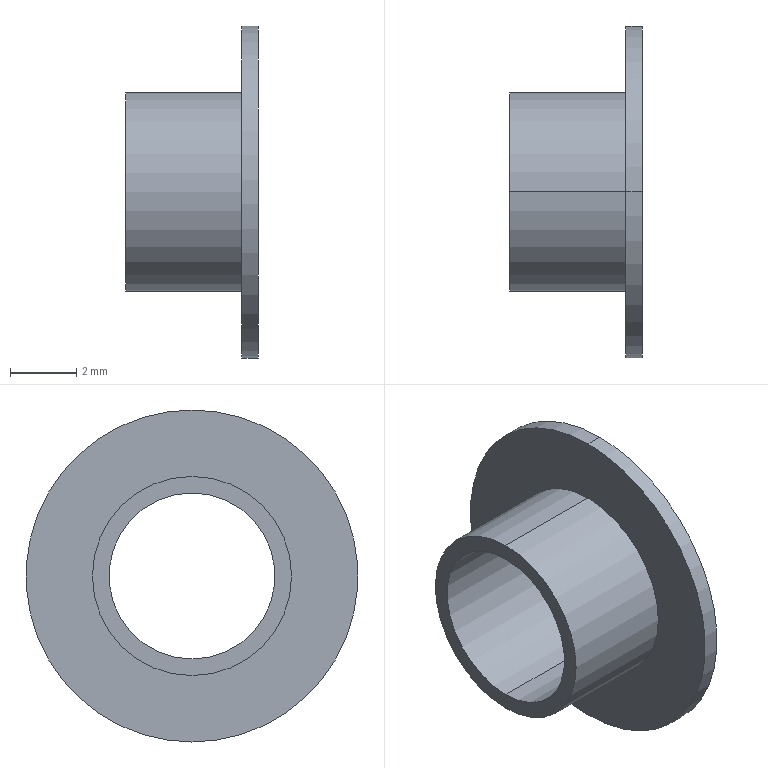Part | SolidWorks | features Revolution 1 | 1 solid | 9 faces | box 4 x 10 x 10 mm | volume 59.69 mm3 | cylinder 6 | plane 3 | commonest cylinder face diameters 5 x2 6 x2 10 x2
STEP:
#1=CARTESIAN_POINT('',(4.,0.,5.));
#2=VERTEX_POINT('',#1);
#3=CARTESIAN_POINT('',(4.,0.,-5.));
#4=VERTEX_POINT('',#3);
#5=CARTESIAN_POINT('',(4.,0.,0.));
#6=DIRECTION('',(-1.,0.,0.));
#7=DIRECTION('',(0.,0.,1.));
#8=AXIS2_PLACEMENT_3D('',#5,#6,#7);
#9=CIRCLE('',#8,5.);
#10=EDGE_CURVE('',#2,#4,#9,.T.);
#11=ORIENTED_EDGE('',*,*,#10,.T.);
#12=CARTESIAN_POINT('',(3.5,0.,-5.));
#13=VERTEX_POINT('',#12);
#14=CARTESIAN_POINT('',(-238.363,0.,-5.));
#15=DIRECTION('',(-1.,0.,0.));
#16=VECTOR('',#15,1000.);
#17=LINE('',#14,#16);
#18=EDGE_CURVE('',#4,#13,#17,.T.);
#19=ORIENTED_EDGE('',*,*,#18,.T.);
#20=CARTESIAN_POINT('',(3.5,0.,5.));
#21=VERTEX_POINT('',#20);
#22=CARTESIAN_POINT('',(3.5,0.,0.));
#23=DIRECTION('',(-1.,0.,0.));
#24=DIRECTION('',(0.,0.,1.));
#25=AXIS2_PLACEMENT_3D('',#22,#23,#24);
#26=CIRCLE('',#25,5.);
#27=EDGE_CURVE('',#21,#13,#26,.T.);
#28=ORIENTED_EDGE('',*,*,#27,.F.);
#29=CARTESIAN_POINT('',(-238.363,0.,5.));
#30=DIRECTION('',(-1.,0.,0.));
#31=VECTOR('',#30,1000.);
#32=LINE('',#29,#31);
#33=EDGE_CURVE('',#2,#21,#32,.T.);
#34=ORIENTED_EDGE('',*,*,#33,.F.);
#35=EDGE_LOOP('',(#11,#19,#28,#34));
#36=FACE_OUTER_BOUND('',#35,.T.);
#37=CARTESIAN_POINT('',(-238.363,0.,0.));
#38=DIRECTION('',(-1.,0.,0.));
#39=DIRECTION('',(0.,0.,1.));
#40=AXIS2_PLACEMENT_3D('',#37,#38,#39);
#41=CYLINDRICAL_SURFACE('',#40,5.);
#42=ADVANCED_FACE('',(#36),#41,.T.);
#43=CARTESIAN_POINT('',(3.5,0.,3.));
#44=VERTEX_POINT('',#43);
#45=CARTESIAN_POINT('',(3.5,0.,-3.));
#46=VERTEX_POINT('',#45);
#47=CARTESIAN_POINT('',(3.5,0.,0.));
#48=DIRECTION('',(-1.,0.,0.));
#49=DIRECTION('',(0.,0.,1.));
#50=AXIS2_PLACEMENT_3D('',#47,#48,#49);
#51=CIRCLE('',#50,3.);
#52=EDGE_CURVE('',#44,#46,#51,.T.);
#53=ORIENTED_EDGE('',*,*,#52,.T.);
#54=CARTESIAN_POINT('',(0.,0.,-3.));
#55=VERTEX_POINT('',#54);
#56=CARTESIAN_POINT('',(-238.363,0.,-3.));
#57=DIRECTION('',(-1.,0.,0.));
#58=VECTOR('',#57,1000.);
#59=LINE('',#56,#58);
#60=EDGE_CURVE('',#46,#55,#59,.T.);
#61=ORIENTED_EDGE('',*,*,#60,.T.);
#62=CARTESIAN_POINT('',(0.,0.,3.));
#63=VERTEX_POINT('',#62);
#64=CARTESIAN_POINT('',(0.,0.,0.));
#65=DIRECTION('',(-1.,0.,0.));
#66=DIRECTION('',(0.,0.,1.));
#67=AXIS2_PLACEMENT_3D('',#64,#65,#66);
#68=CIRCLE('',#67,3.);
#69=EDGE_CURVE('',#63,#55,#68,.T.);
#70=ORIENTED_EDGE('',*,*,#69,.F.);
#71=CARTESIAN_POINT('',(-238.363,0.,3.));
#72=DIRECTION('',(-1.,0.,0.));
#73=VECTOR('',#72,1000.);
#74=LINE('',#71,#73);
#75=EDGE_CURVE('',#44,#63,#74,.T.);
#76=ORIENTED_EDGE('',*,*,#75,.F.);
#77=EDGE_LOOP('',(#53,#61,#70,#76));
#78=FACE_OUTER_BOUND('',#77,.T.);
#79=CARTESIAN_POINT('',(-238.363,0.,0.));
#80=DIRECTION('',(-1.,0.,0.));
#81=DIRECTION('',(0.,0.,1.));
#82=AXIS2_PLACEMENT_3D('',#79,#80,#81);
#83=CYLINDRICAL_SURFACE('',#82,3.);
#84=ADVANCED_FACE('',(#78),#83,.T.);
#85=CARTESIAN_POINT('',(4.,0.,-2.5));
#86=VERTEX_POINT('',#85);
#87=CARTESIAN_POINT('',(4.,0.,2.5));
#88=VERTEX_POINT('',#87);
#89=CARTESIAN_POINT('',(4.,0.,0.));
#90=DIRECTION('',(-1.,0.,0.));
#91=DIRECTION('',(0.,0.,1.));
#92=AXIS2_PLACEMENT_3D('',#89,#90,#91);
#93=CIRCLE('',#92,2.5);
#94=EDGE_CURVE('',#86,#88,#93,.T.);
#95=ORIENTED_EDGE('',*,*,#94,.F.);
#96=CARTESIAN_POINT('',(0.,0.,-2.5));
#97=VERTEX_POINT('',#96);
#98=CARTESIAN_POINT('',(-238.363,0.,-2.5));
#99=DIRECTION('',(-1.,0.,0.));
#100=VECTOR('',#99,1000.);
#101=LINE('',#98,#100);
#102=EDGE_CURVE('',#86,#97,#101,.T.);
#103=ORIENTED_EDGE('',*,*,#102,.T.);
#104=CARTESIAN_POINT('',(0.,0.,2.5));
#105=VERTEX_POINT('',#104);
#106=CARTESIAN_POINT('',(0.,0.,0.));
#107=DIRECTION('',(-1.,0.,0.));
#108=DIRECTION('',(0.,0.,1.));
#109=AXIS2_PLACEMENT_3D('',#106,#107,#108);
#110=CIRCLE('',#109,2.5);
#111=EDGE_CURVE('',#97,#105,#110,.T.);
#112=ORIENTED_EDGE('',*,*,#111,.T.);
#113=CARTESIAN_POINT('',(-238.363,0.,2.5));
#114=DIRECTION('',(-1.,0.,0.));
#115=VECTOR('',#114,1000.);
#116=LINE('',#113,#115);
#117=EDGE_CURVE('',#88,#105,#116,.T.);
#118=ORIENTED_EDGE('',*,*,#117,.F.);
#119=EDGE_LOOP('',(#95,#103,#112,#118));
#120=FACE_OUTER_BOUND('',#119,.T.);
#121=CARTESIAN_POINT('',(-238.363,0.,0.));
#122=DIRECTION('',(-1.,0.,0.));
#123=DIRECTION('',(0.,0.,1.));
#124=AXIS2_PLACEMENT_3D('',#121,#122,#123);
#125=CYLINDRICAL_SURFACE('',#124,2.5);
#126=ADVANCED_FACE('',(#120),#125,.F.);
#127=ORIENTED_EDGE('',*,*,#102,.F.);
#128=CARTESIAN_POINT('',(4.,0.,0.));
#129=DIRECTION('',(-1.,0.,0.));
#130=DIRECTION('',(0.,0.,1.));
#131=AXIS2_PLACEMENT_3D('',#128,#129,#130);
#132=CIRCLE('',#131,2.5);
#133=EDGE_CURVE('',#88,#86,#132,.T.);
#134=ORIENTED_EDGE('',*,*,#133,.F.);
#135=ORIENTED_EDGE('',*,*,#117,.T.);
#136=CARTESIAN_POINT('',(0.,0.,0.));
#137=DIRECTION('',(-1.,0.,0.));
#138=DIRECTION('',(0.,0.,1.));
#139=AXIS2_PLACEMENT_3D('',#136,#137,#138);
#140=CIRCLE('',#139,2.5);
#141=EDGE_CURVE('',#105,#97,#140,.T.);
#142=ORIENTED_EDGE('',*,*,#141,.T.);
#143=EDGE_LOOP('',(#127,#134,#135,#142));
#144=FACE_OUTER_BOUND('',#143,.T.);
#145=CARTESIAN_POINT('',(-238.363,0.,0.));
#146=DIRECTION('',(-1.,0.,0.));
#147=DIRECTION('',(0.,0.,1.));
#148=AXIS2_PLACEMENT_3D('',#145,#146,#147);
#149=CYLINDRICAL_SURFACE('',#148,2.5);
#150=ADVANCED_FACE('',(#144),#149,.F.);
#151=ORIENTED_EDGE('',*,*,#141,.F.);
#152=ORIENTED_EDGE('',*,*,#111,.F.);
#153=EDGE_LOOP('',(#151,#152));
#154=FACE_BOUND('',#153,.T.);
#155=ORIENTED_EDGE('',*,*,#69,.T.);
#156=CARTESIAN_POINT('',(0.,0.,0.));
#157=DIRECTION('',(-1.,0.,0.));
#158=DIRECTION('',(0.,0.,1.));
#159=AXIS2_PLACEMENT_3D('',#156,#157,#158);
#160=CIRCLE('',#159,3.);
#161=EDGE_CURVE('',#55,#63,#160,.T.);
#162=ORIENTED_EDGE('',*,*,#161,.T.);
#163=EDGE_LOOP('',(#155,#162));
#164=FACE_OUTER_BOUND('',#163,.T.);
#165=CARTESIAN_POINT('',(0.,0.,-2.5));
#166=DIRECTION('',(1.,0.,0.));
#167=DIRECTION('',(0.,0.,-1.));
#168=AXIS2_PLACEMENT_3D('',#165,#166,#167);
#169=PLANE('',#168);
#170=ADVANCED_FACE('',(#154,#164),#169,.F.);
#171=ORIENTED_EDGE('',*,*,#60,.F.);
#172=CARTESIAN_POINT('',(3.5,0.,0.));
#173=DIRECTION('',(-1.,0.,0.));
#174=DIRECTION('',(0.,0.,1.));
#175=AXIS2_PLACEMENT_3D('',#172,#173,#174);
#176=CIRCLE('',#175,3.);
#177=EDGE_CURVE('',#46,#44,#176,.T.);
#178=ORIENTED_EDGE('',*,*,#177,.T.);
#179=ORIENTED_EDGE('',*,*,#75,.T.);
#180=ORIENTED_EDGE('',*,*,#161,.F.);
#181=EDGE_LOOP('',(#171,#178,#179,#180));
#182=FACE_OUTER_BOUND('',#181,.T.);
#183=CARTESIAN_POINT('',(-238.363,0.,0.));
#184=DIRECTION('',(-1.,0.,0.));
#185=DIRECTION('',(0.,0.,1.));
#186=AXIS2_PLACEMENT_3D('',#183,#184,#185);
#187=CYLINDRICAL_SURFACE('',#186,3.);
#188=ADVANCED_FACE('',(#182),#187,.T.);
#189=ORIENTED_EDGE('',*,*,#52,.F.);
#190=ORIENTED_EDGE('',*,*,#177,.F.);
#191=EDGE_LOOP('',(#189,#190));
#192=FACE_BOUND('',#191,.T.);
#193=ORIENTED_EDGE('',*,*,#27,.T.);
#194=CARTESIAN_POINT('',(3.5,0.,0.));
#195=DIRECTION('',(-1.,0.,0.));
#196=DIRECTION('',(0.,0.,1.));
#197=AXIS2_PLACEMENT_3D('',#194,#195,#196);
#198=CIRCLE('',#197,5.);
#199=EDGE_CURVE('',#13,#21,#198,.T.);
#200=ORIENTED_EDGE('',*,*,#199,.T.);
#201=EDGE_LOOP('',(#193,#200));
#202=FACE_OUTER_BOUND('',#201,.T.);
#203=CARTESIAN_POINT('',(3.5,0.,-3.));
#204=DIRECTION('',(1.,0.,0.));
#205=DIRECTION('',(0.,0.,-1.));
#206=AXIS2_PLACEMENT_3D('',#203,#204,#205);
#207=PLANE('',#206);
#208=ADVANCED_FACE('',(#192,#202),#207,.F.);
#209=ORIENTED_EDGE('',*,*,#18,.F.);
#210=CARTESIAN_POINT('',(4.,0.,0.));
#211=DIRECTION('',(-1.,0.,0.));
#212=DIRECTION('',(0.,0.,1.));
#213=AXIS2_PLACEMENT_3D('',#210,#211,#212);
#214=CIRCLE('',#213,5.);
#215=EDGE_CURVE('',#4,#2,#214,.T.);
#216=ORIENTED_EDGE('',*,*,#215,.T.);
#217=ORIENTED_EDGE('',*,*,#33,.T.);
#218=ORIENTED_EDGE('',*,*,#199,.F.);
#219=EDGE_LOOP('',(#209,#216,#217,#218));
#220=FACE_OUTER_BOUND('',#219,.T.);
#221=CARTESIAN_POINT('',(-238.363,0.,0.));
#222=DIRECTION('',(-1.,0.,0.));
#223=DIRECTION('',(0.,0.,1.));
#224=AXIS2_PLACEMENT_3D('',#221,#222,#223);
#225=CYLINDRICAL_SURFACE('',#224,5.);
#226=ADVANCED_FACE('',(#220),#225,.T.);
#227=ORIENTED_EDGE('',*,*,#10,.F.);
#228=ORIENTED_EDGE('',*,*,#215,.F.);
#229=EDGE_LOOP('',(#227,#228));
#230=FACE_OUTER_BOUND('',#229,.T.);
#231=ORIENTED_EDGE('',*,*,#133,.T.);
#232=ORIENTED_EDGE('',*,*,#94,.T.);
#233=EDGE_LOOP('',(#231,#232));
#234=FACE_BOUND('',#233,.T.);
#235=CARTESIAN_POINT('',(4.,0.,-5.));
#236=DIRECTION('',(-1.,0.,0.));
#237=DIRECTION('',(0.,0.,1.));
#238=AXIS2_PLACEMENT_3D('',#235,#236,#237);
#239=PLANE('',#238);
#240=ADVANCED_FACE('',(#230,#234),#239,.F.);
#241=CLOSED_SHELL('',(#42,#84,#126,#150,#170,#188,#208,#226,#240));
#242=MANIFOLD_SOLID_BREP('',#241);
#243=CARTESIAN_POINT('',(0.,0.,0.));
#244=DIRECTION('',(0.,0.,1.));
#245=DIRECTION('',(1.,0.,0.));
#246=AXIS2_PLACEMENT_3D('',#243,#244,#245);
#247=(LENGTH_UNIT()NAMED_UNIT(*)SI_UNIT(.MILLI.,.METRE.));
#248=UNCERTAINTY_MEASURE_WITH_UNIT(LENGTH_MEASURE(0.00001),#247,'','');
#249=(NAMED_UNIT(*)PLANE_ANGLE_UNIT()SI_UNIT($,.RADIAN.));
#250=(NAMED_UNIT(*)SI_UNIT($,.STERADIAN.)SOLID_ANGLE_UNIT());
#251=(GEOMETRIC_REPRESENTATION_CONTEXT(3)GLOBAL_UNCERTAINTY_ASSIGNED_CONTEXT((#248))GLOBAL_UNIT_ASSIGNED_CONTEXT((#247,#249,#250))REPRESENTATION_CONTEXT('',''));
#252=ADVANCED_BREP_SHAPE_REPRESENTATION('',(#242,#246),#251);